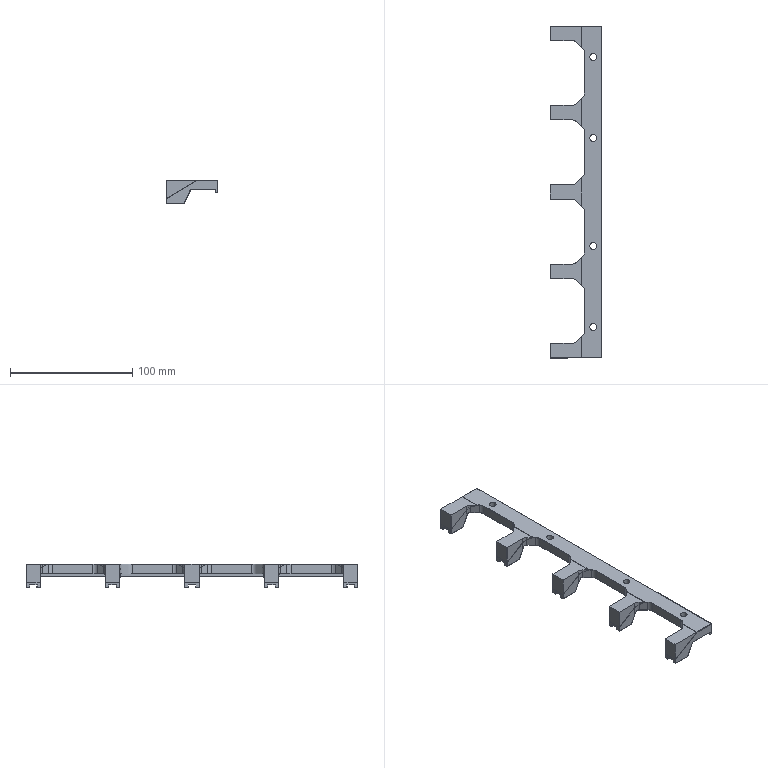Part | 2 solids | 470 faces | box 42 x 271.8 x 19 mm | volume 99365 mm3 | plane 384 | cylinder 54 | cone 32 | commonest cylinder face diameters 10 x32 5.5 x8 26.419 x8 26.46 x6